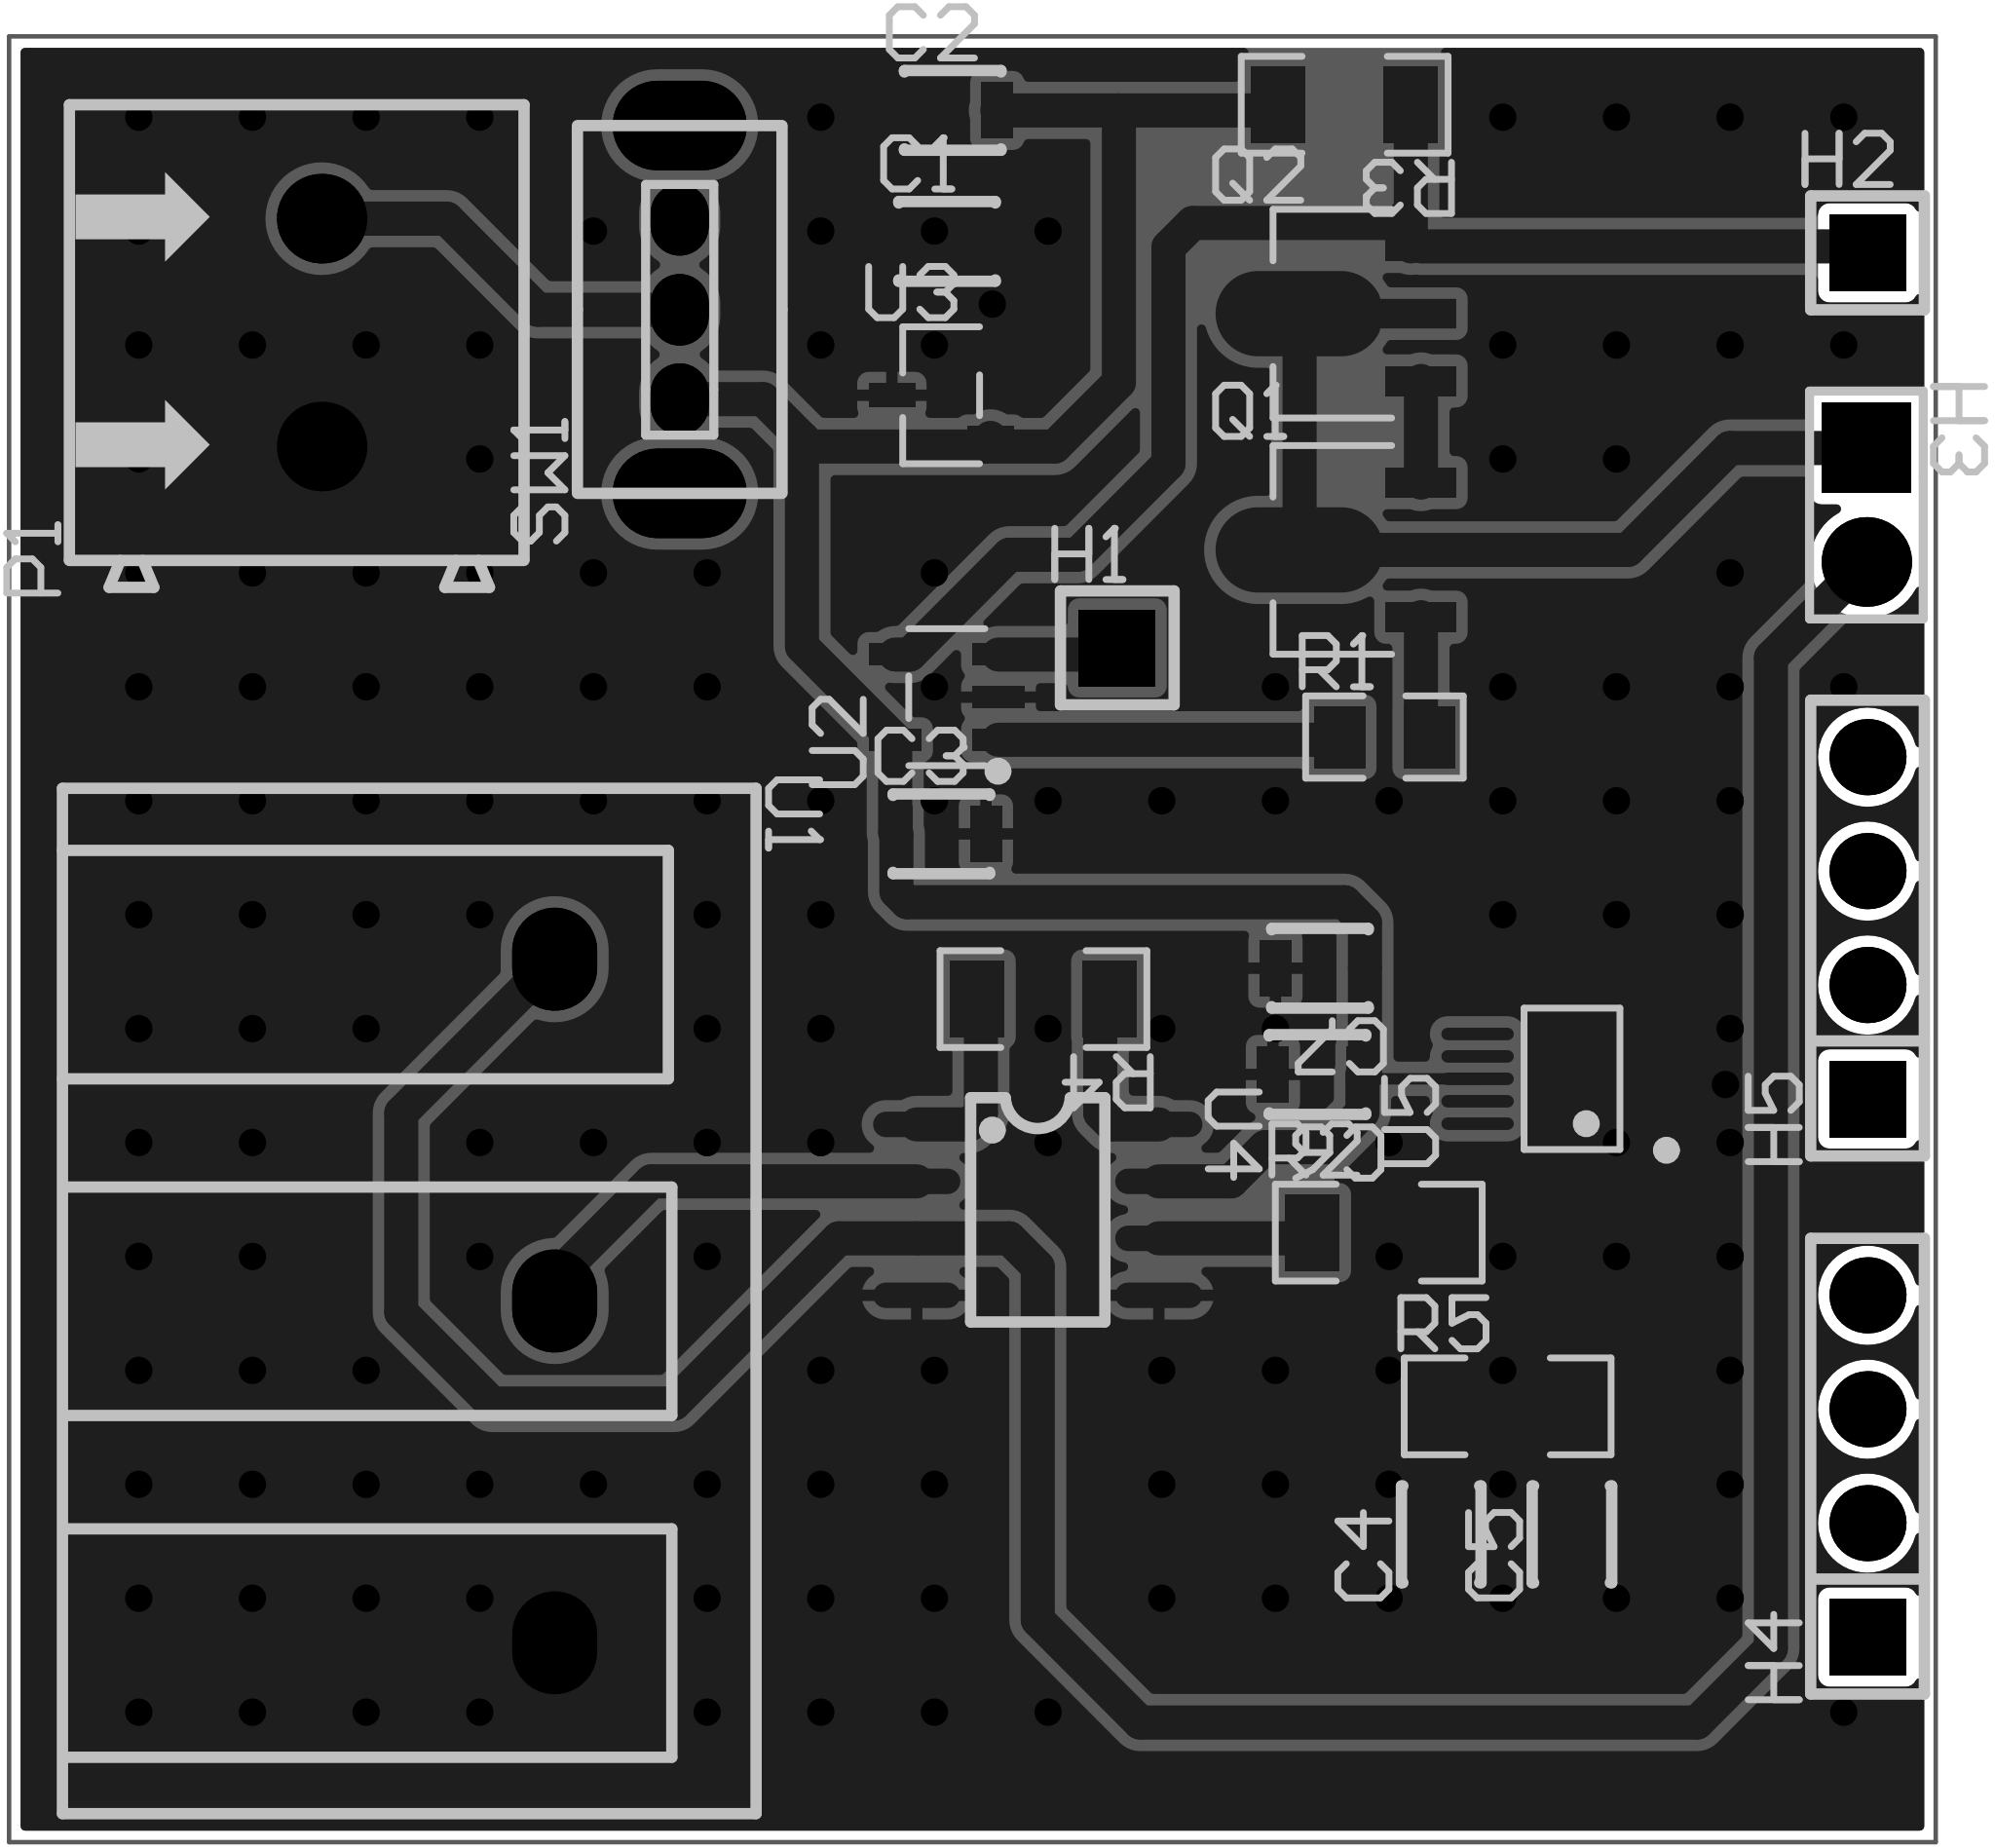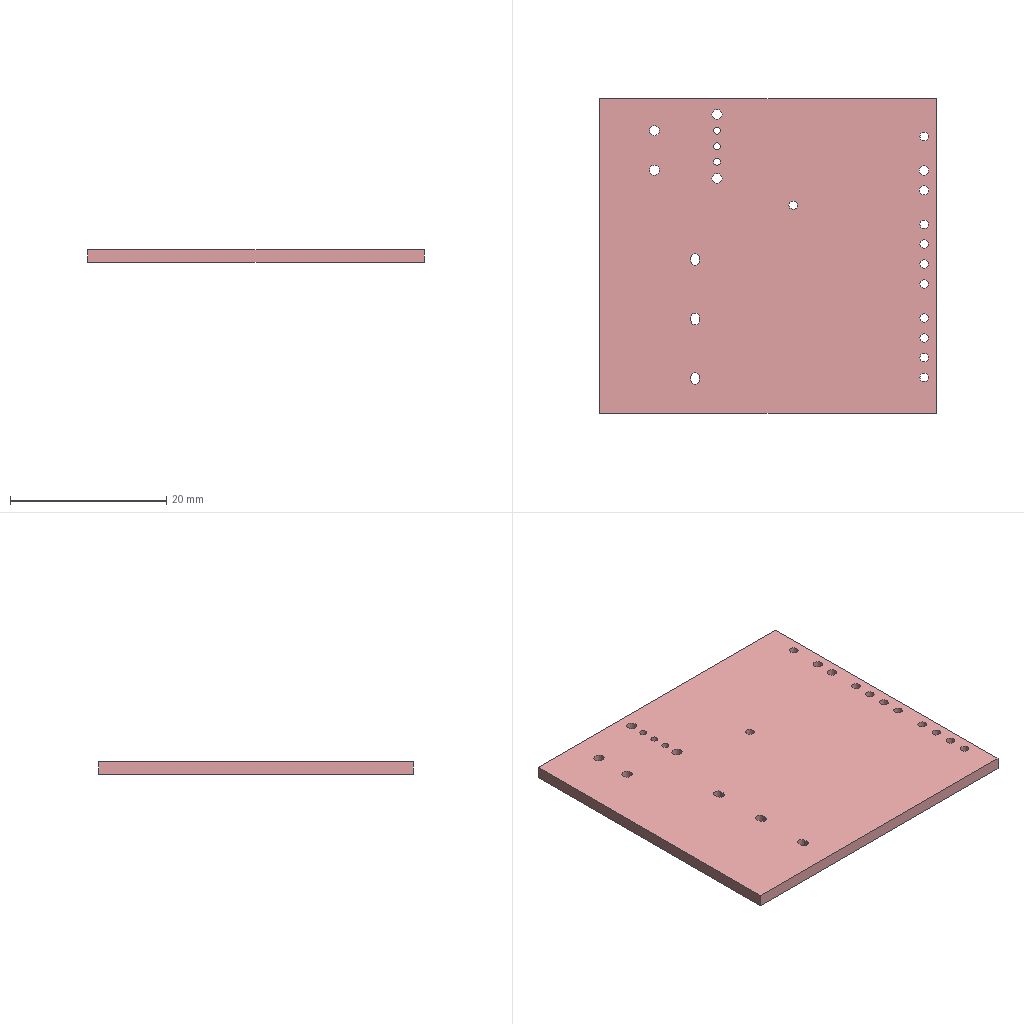Circuit board layout | Altium Designer | box 43.1 x 40.3 x 1.6 mm
Layer stack:
# Altium Designer layer stack of  (unit mm; dielectric type: 0 none, 1 core, 2 prepreg, 3 surface material)
index,name,kind,layer,copper_thickness_mm,dielectric_type,dielectric_thickness_mm,dielectric_material,dielectric_constant
0,Top Paste Mask Layer,other,,,,,,
1,Top Silkscreen Layer,other,,,,,,
2,Top Solder Mask Layer,dielectric,,,3,0.01,,3.3
3,Top Layer,copper,Top Layer,0.035,,,,
4,Dielectric1,dielectric,,,3,1.51,FR4,4.5
5,Bottom Layer,copper,Bottom Layer,0.035,,,,
6,Bottom Solder Mask Layer,dielectric,,,3,0.01,,3.3
7,Bottom Silkscreen Layer,other,,,,,,
8,Bottom Paste Mask Layer,other,,,,,,
# drill layer pairs: low layer,high layer
drill_pair,Top Layer,Bottom Layer
Part placement:
Designator,Comment,Layer,Footprint,Center-X(mm),Center-Y(mm),Rotation
C1,100nF,TopLayer,CAP-SMD_L2.0-W1.25,105.283,119.888,0
P1,WJ500V-5.08-2P,TopLayer,CONN-TH_2P-P5.00_WJ500V-5.08-2P,91.313,117.856,90
C2,100nF,TopLayer,CAP-SMD_L2.0-W1.25,105.41,122.809,0
C3,100nF,TopLayer,CAP-SMD_L2.0-W1.25,105.156,106.68,0
C4,1uF,TopLayer,CAP-SMD_L2.0-W1.25,116.332,91.059,90
C5,4.7nf,TopLayer,CAP-SMD_L2.0-W1.25,119.253,91.059,90
C6,100nf,TopLayer,CAP-SMD_L2.0-W1.25,113.57,101.316,180
C7,100nf,TopLayer,CAP-SMD_L2.0-W1.25,113.627,103.685,180
H1,PZ254V-11-01P,TopLayer,HDR-TH_1P-P2.54-V-M,109.092,110.827,0
H2,PZ254V-11-01P,TopLayer,HDR-TH_1P-P2.54-V-M,125.857,119.634,0
H3,PZ254V-11-02P,TopLayer,HDR-TH_2P-P2.54-V-M,125.832,114.012,270
H4,PZ254V-11-04P,TopLayer,HDR-TH_4P-P2.54-V-M,125.857,92.583,90
H5,PZ254V-11-04P,TopLayer,HDR-TH_4P-P2.54-V-M,125.857,104.58,90
Q1,2SA1201,TopLayer,SOT-89-3_L4.5-W2.5-P1.50-LS4.2-BR,114.717,113.011,0
Q2,2SA1201,TopLayer,SOT-89-3_L4.5-W2.5-P1.50-LS4.2-BR,114.717,118.278,0
R1,10kΩ,TopLayer,R0805,115.062,108.839,0
R2,1KΩ,TopLayer,R1206,114.935,97.79,0
R3,2.7KΩ,TopLayer,R1206,114.173,122.936,180
R4,6KΩ,TopLayer,R1206,107.442,102.997,180
R5,1KΩ,TopLayer,R1206,117.815,93.917,0
U1,JL762-76203BA1,TopLayer,CONN-TH_JL762-76203BA1,96.52,96.266,270
U2,SGM8551XN5G/TR,TopLayer,SOT-23-5_L3.0-W1.7-P0.95-LS2.8-BL,105.283,109.728,90
U3,REF3025AIDBZT,TopLayer,SOT-23-3_L3.0-W1.7-P0.95-LS2.9-BR,105.156,116.459,0
U4,AD623ARZ-R7,TopLayer,SOIC-8_L5.0-W4.0-P1.27-LS6.0-BL,107.315,98.298,270
U5,GD30AD3344,TopLayer,MSOP-10_L3.0-W3.0-P0.50-LS5.0-BL,119.253,101.219,90
SW1,,TopLayer,拨动开关,99.314,118.372,90
Pad and via stacks:
# Altium Designer via and pad stacks of  (unit mm). Each distinct definition once, with the count of objects using it.
# via: kind,start_layer,end_layer,hole_mm,diameter_mm,mode(0 simple;1 top-mid-bottom;2 full stack),diameter_per_layer,count,example_net
# pad: kind,layer,hole_mm,hole_type(0 round;1 square;2 slot),plating,top_size,top_shape(1 round;2 rect;3 octagon;9 rounded rect),mid_size,bottom_size,mode,footprint,size_per_layer,count,example
pad,Top Layer,0,0,plated,1.25x0.7,2,1.25x0.7,1.25x0.7,0,CAP-SMD_L2.0-W1.25,,14,C1.1
pad,Top Layer,0,0,plated,1.575x0.672,2,1.575x0.672,1.575x0.672,0,SOT-89-3_L4.5-W2.5-P1.50-LS4.2-BR,,4,Q1.1
pad,Top Layer,0,0,plated,0.95x0.95,1,0.95x0.95,0.95x0.95,0,SOT-89-3_L4.5-W2.5-P1.50-LS4.2-BR,,2,Q1.2
pad,Top Layer,0,0,plated,1.133x1.377,2,1.133x1.377,1.133x1.377,0,R0805,,2,R1.2
pad,Top Layer,0,0,plated,1.208x1.701,2,1.208x1.701,1.208x1.701,0,R1206,,8,R2.2
pad,Top Layer,0,0,plated,0.49x1.157,2,0.49x1.157,0.49x1.157,0,SOT-23-5_L3.0-W1.7-P0.95-LS2.8-BL,,3,U2.1
pad,Top Layer,0,0,plated,0.49x1.175,2,0.49x1.175,0.49x1.175,0,SOT-23-5_L3.0-W1.7-P0.95-LS2.8-BL,,2,U2.4
pad,Top Layer,0,0,plated,1.038x0.532,2,1.038x0.532,1.038x0.532,0,SOT-23-3_L3.0-W1.7-P0.95-LS2.9-BR,,3,U3.1
pad,Top Layer,0,0,plated,0.5684x1.95,1,0.5684x1.95,0.5684x1.95,0,SOIC-8_L5.0-W4.0-P1.27-LS6.0-BL,,8,U4.1
pad,Top Layer,0,0,plated,0.28x1.62,1,0.28x1.62,0.28x1.62,0,MSOP-10_L3.0-W3.0-P0.50-LS5.0-BL,,10,U5.1
pad,Multi-Layer,1.3,0,plated,2x2,1,2x2,2x2,0,CONN-TH_2P-P5.00_WJ500V-5.08-2P,,2,P1.2
pad,Multi-Layer,1.1,0,plated,1.7x1.7,2,1.7x1.7,1.7x1.7,0,HDR-TH_1P-P2.54-V-M,,2,H1.1
pad,Multi-Layer,1.2,0,plated,2x2,2,2x2,2x2,0,HDR-TH_2P-P2.54-V-M,,1,H3.1
pad,Multi-Layer,1.2,0,plated,2x2,1,2x2,2x2,0,HDR-TH_2P-P2.54-V-M,,1,H3.2
pad,Multi-Layer,1.1,0,plated,1.7x1.7,2,1.7x1.7,1.7x1.7,0,HDR-TH_4P-P2.54-V-M,,2,H4.1
pad,Multi-Layer,1.1,0,plated,1.7x1.7,1,1.7x1.7,1.7x1.7,0,HDR-TH_4P-P2.54-V-M,,6,H4.2
pad,Multi-Layer,1.1,2,plated,2.3x1.9,1,2.3x1.9,2.3x1.9,0,CONN-TH_JL762-76203BA1,,3,U1.1
pad,Multi-Layer,0.8992,0,plated,1.6x1.3,1,1.6x1.3,1.6x1.3,0,\u00B2\u00A6\u00B6\u00AF\u00BF\u00AA\u00B9\u00D8,,3,SW1.1
pad,Multi-Layer,1.3,0,plated,3x1.999,1,3x1.999,3x1.999,0,\u00B2\u00A6\u00B6\u00AF\u00BF\u00AA\u00B9\u00D8,,2,SW1.4
via,Top Layer,Bottom Layer,0.3048,0.61,0,,146,$1N4
Copper pours:
name,layer,net,type(0 solid;1 hatched;2 none)
Top Layer-GND,Top Layer,GND,0
Bottom Layer-GND,Bottom Layer,GND,0